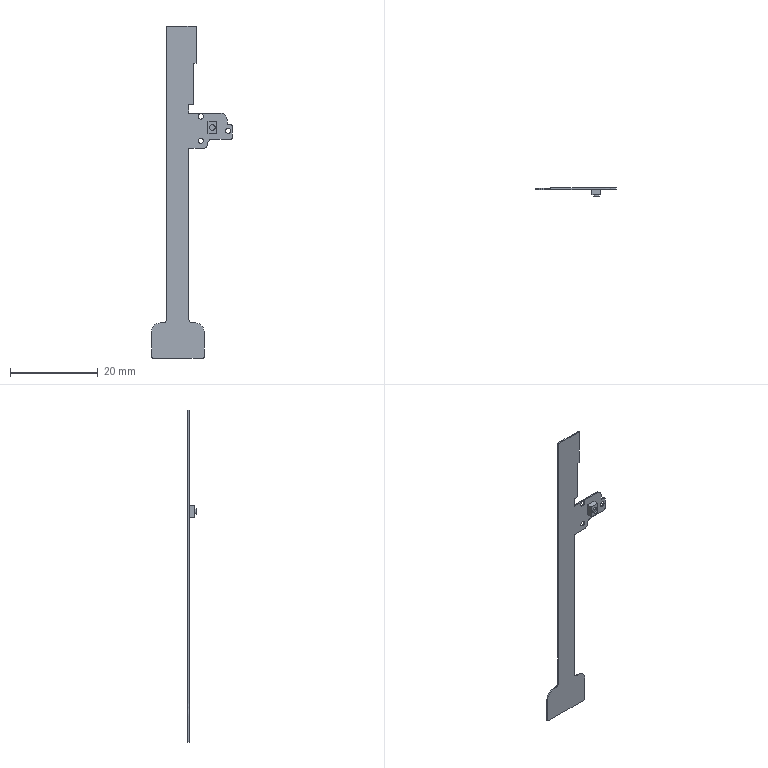Part | Creo | 1 solid | 46 faces | box 18.5 x 1.9 x 75.87 mm | volume 163.267 mm3 | plane 27 | cylinder 19 | commonest cylinder face diameters 1.2 x6 0.4 x2 1 x2 1.3 x2 1.9 x2 2 x2